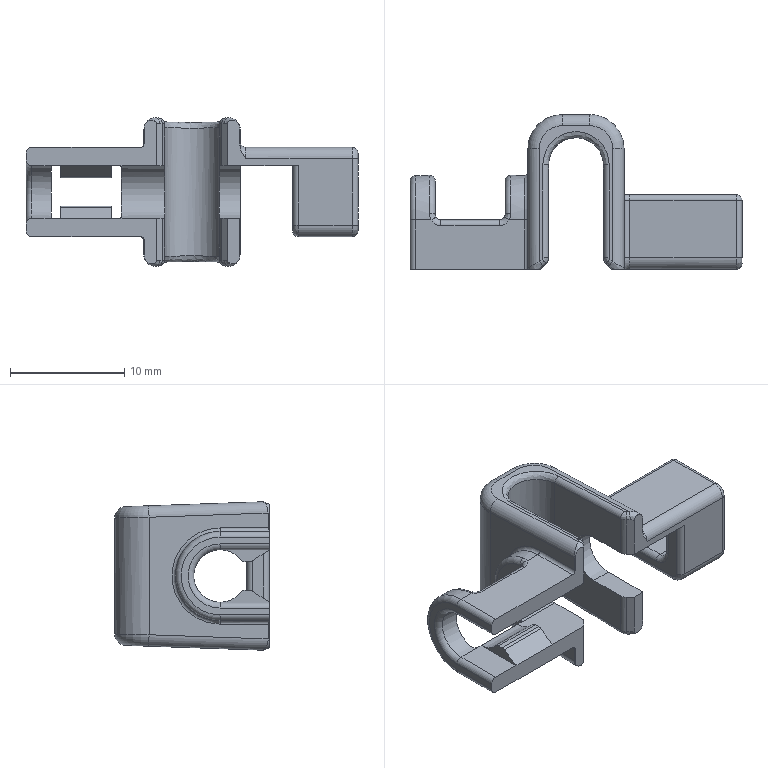Part | STEP file | ZXW735-L-175_2_1_1 | 1 solid | 159 faces | box 29 x 13.5 x 12.958 mm | volume 1025 mm3 | cylinder 70 | plane 44 | spline 20 | torus 19 | sphere 6 | commonest cylinder face diameters 1 x44 2 x10 4.6 x5 1.4 x4 0.6 x2 6 x2